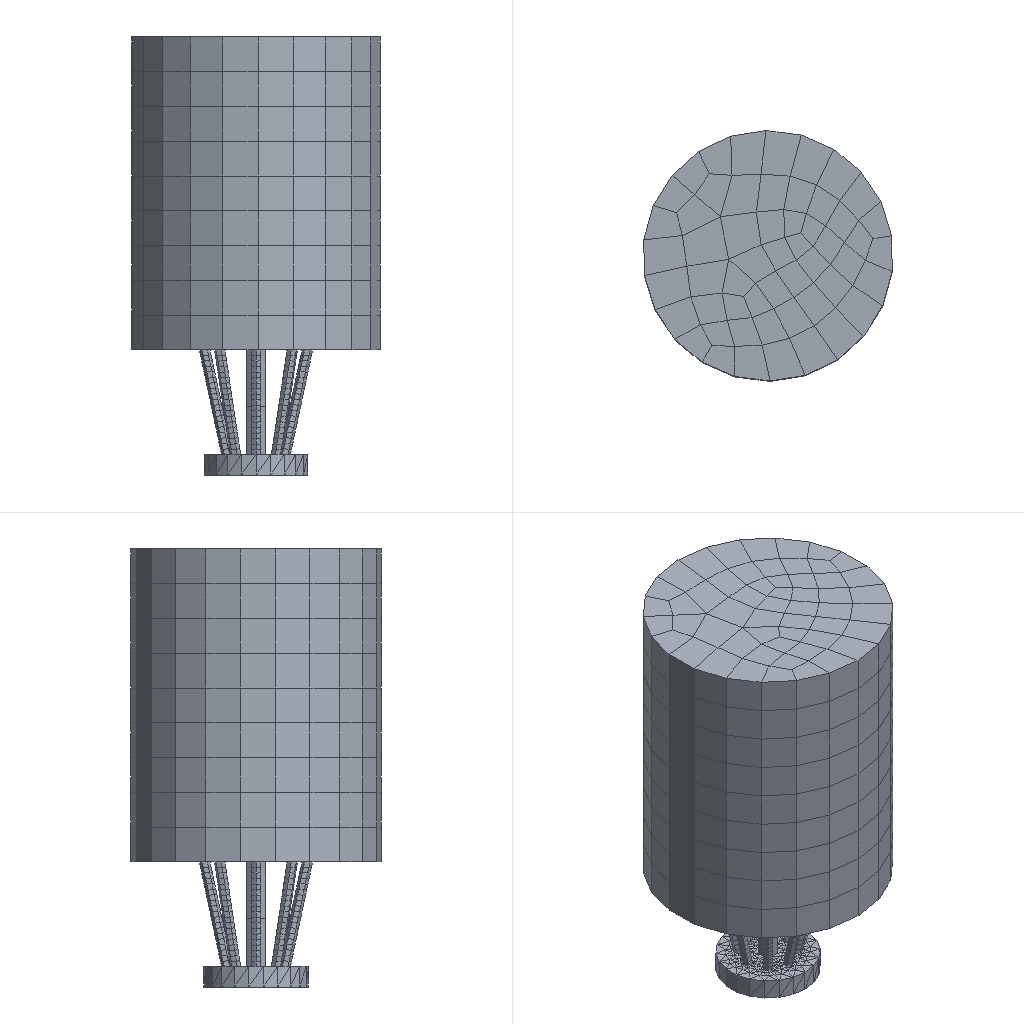Simulation study | abaqus
Set-up summary:
category,name,step,type,value,unit,region
solver,abaqus
solver,version,,,Abaqus/Standard 2020
units,not stated in the deck,,not stated
analysis,deck,,static,static
load_step,Step-1,Step-1,static
load_step,requested,,,1
mesh,nodes,,,8569
mesh,elements,,,4242
element_type,C3D8,,solid,1718
element_type,C3D10,,solid,2524
load,load commands in deck,,count,2
bc,support commands in deck,,count,3
material,CON,,in results
material,SOIL,,in results
check,setup vs results,,match,"per instance, exact: element labels, types and connectivity; labels of the nodes the elements use; coordinates of those nodes at SINGLE_PRECISION in 2 of 3 instance(s)"
Abaqus input file, long lists of numbers shortened:
*Heading
** Job name: Job-2 Model name: Model-2
** Generated by: Abaqus/CAE 2020
*Preprint, echo=NO, model=NO, history=NO, contact=NO
**
** PARTS
**
*Part, name=Part-3
*Node
      1,   3.383,  -3.971,          12.
      2,   1.788,  -2.376,   1.388
** (3727 more lines like these left out)
*Element, type=C3D8
 1, 174, 173, 172, 169,   1,  36,  35,  32
 2, 172, 171, 170, 169,  35,  34,  33,  32
** (1230 more lines like these left out)
*Nset, nset=Set-2, generate
    1,  3729,     1
*Elset, elset=Set-2, generate
    1,  1232,     1
** Section: con
*Solid Section, elset=Set-2, material=con
,
*End Part
**
*Part, name=cut-chengtai
*Node
      1,   1.788,  -2.376,   1.388
      2,  -2.376,  -1.788,   1.388
** (4178 more lines like these left out)
*Element, type=C3D10
   1,  398,  158,  399,  400,  634,  633,  632,  636,  635,  637
   2,  401,  402,  302,  403,  640,  639,  638,  642,  641,  643
** (2522 more lines like these left out)
*Nset, nset=Set-4, generate
    1,  4180,     1
*Elset, elset=Set-4, generate
    1,  2524,     1
** Section: con
*Solid Section, elset=Set-4, material=con
,
*End Part
**
*Part, name=soil
*Node
      1,   9.2,   -7.705,           0.
      2,   10.998,   -4.801,           0.
** (658 more lines like these left out)
*Element, type=C3D8
  1,  89,  86,  85,  90,  23,  20,  19,  24
  2,  90,  85,  84,  91,  24,  19,  18,  25
** (484 more lines like these left out)
*Nset, nset=Set-2, generate
   1,  660,    1
*Elset, elset=Set-2, generate
   1,  486,    1
** Section: soil
*Solid Section, elset=Set-2, material=soil
,
*End Part
**
**
** ASSEMBLY
**
*Assembly, name=Assembly
**
*Instance, name=soil-1, part=soil
          0.,           0.,          12.
*End Instance
**
*Instance, name=cut-chengtai-1, part=cut-chengtai
*End Instance
**
*Instance, name=Part-3-1, part=Part-3
*End Instance
**
*Nset, nset=Set-3, instance=soil-1, generate
 595,  660,    1
*Elset, elset=Set-3, instance=soil-1, generate
 433,  486,    1
*Nset, nset=Set-4, instance=soil-1
   1,   2,   3,   4,   5,   6,   7,   8,   9,  10,  11,  12,  13,  14,  15,  16
  17,  18,  19,  20,  21,  22,  67,  68,  69,  70,  71,  72,  73,  74,  75,  76
** (12 more lines like these left out)
*Elset, elset=Set-4, instance=soil-1
   1,   2,   3,   4,  13,  14,  15,  16,  17,  18,  19,  20,  22,  23,  24,  25
  26,  27,  28,  29,  48,  49,  55,  56,  57,  58,  67,  68,  69,  70,  71,  72
** (11 more lines like these left out)
*Nset, nset=Set-5, instance=soil-1, generate
 595,  660,    1
*Elset, elset=Set-5, instance=soil-1, generate
 433,  486,    1
*Nset, nset=m_Set-1, instance=Part-3-1
    1,    3,    4,    6,    7,   10,   11,   13,   14,   17,   18,   20,   21,   24,   25,   27
   28,   31,   32,   33,   34,   35,   36,   42,   43,   44,   45,   46,   47,   48,   49,   50
** (170 more lines like these left out)
*Elset, elset=m_Set-1, instance=Part-3-1
   41,   42,   43,   44,   45,   46,   47,   48,   49,   50,   51,   52,   53,   54,   55,   56
   57,   58,   59,   60,   61,   62,   63,   64,   65,   66,   67,   68,   69,   70,   71,   72
** (55 more lines like these left out)
*Nset, nset=s_Set-1, instance=soil-1, generate
   1,  660,    1
*Elset, elset=s_Set-1, instance=soil-1, generate
   1,  486,    1
*Elset, elset=_Surf-3_S1, internal, instance=cut-chengtai-1
  121, 1557, 1809
*Elset, elset=_Surf-3_S3, internal, instance=cut-chengtai-1
  487,  520,  610,  668,  694,  706,  761,  783,  858,  877,  881,  905,  949, 1073, 1092, 1116
 1209, 1248, 1259, 1293, 1321, 1361, 1389, 1441, 1450, 1472, 1490, 1537, 1539, 1556, 1562, 1566
** (3 more lines like these left out)
*Elset, elset=_Surf-3_S4, internal, instance=cut-chengtai-1
  587,  760, 1074, 1144, 1316, 1449, 1597, 1672, 2343
*Elset, elset=_Surf-3_S2, internal, instance=cut-chengtai-1
  673,  988, 1451, 1619, 1629, 1923, 2221, 2301
*Surface, type=ELEMENT, name=Surf-3
_Surf-3_S1, S1
_Surf-3_S3, S3
_Surf-3_S4, S4
_Surf-3_S2, S2
*Elset, elset=_Surf-4_S3, internal, instance=Part-3-1
    1,    2,    3,    4,    5,    6,    7,    8,    9,   10,   11,   12,   13,   14,   15,   16
   17,   18,   19,   20,   21,   22,   23,   24,   25,   26,   27,   28,   29,   30,   31,   32
** (19 more lines like these left out)
*Elset, elset=_Surf-4_S4, internal, instance=Part-3-1
    1,    2,    3,    4,    5,    6,    7,    8,    9,   10,   11,   12,   13,   14,   15,   16
   17,   18,   19,   20,   21,   22,   23,   24,   25,   26,   27,   28,   29,   30,   31,   32
** (14 more lines like these left out)
*Elset, elset=_Surf-4_S6, internal, instance=Part-3-1
    1,    3,    5,    7,    9,   11,   13,   15,   17,   19,   21,   23,   25,   27,   29,   31
   33,   35,   37,   39,  151,  153,  155,  157,  183,  184,  185,  186,  187,  188,  189,  190
** (14 more lines like these left out)
*Elset, elset=_Surf-4_S5, internal, instance=Part-3-1
    2,    4,    6,    8,   10,   12,   14,   16,   18,   20,   22,   24,   26,   28,   30,   32
   34,   36,   38,   40,  152,  154,  156,  158,  183,  185,  187,  189,  191,  193,  195,  197
** (9 more lines like these left out)
*Surface, type=ELEMENT, name=Surf-4
_Surf-4_S3, S3
_Surf-4_S4, S4
_Surf-4_S6, S6
_Surf-4_S5, S5
*Elset, elset=_m_Surf-1_S3, internal, instance=Part-3-1
    1,    2,    3,    4,    5,    6,    7,    8,    9,   10,   11,   12,   13,   14,   15,   16
   17,   18,   19,   20,   21,   22,   23,   24,   25,   26,   27,   28,   29,   30,   31,   32
** (19 more lines like these left out)
*Elset, elset=_m_Surf-1_S4, internal, instance=Part-3-1
    1,    2,    3,    4,    5,    6,    7,    8,    9,   10,   11,   12,   13,   14,   15,   16
   17,   18,   19,   20,   21,   22,   23,   24,   25,   26,   27,   28,   29,   30,   31,   32
** (14 more lines like these left out)
*Elset, elset=_m_Surf-1_S6, internal, instance=Part-3-1
    1,    3,    5,    7,    9,   11,   13,   15,   17,   19,   21,   23,   25,   27,   29,   31
   33,   35,   37,   39,  151,  153,  155,  157,  183,  184,  185,  186,  187,  188,  189,  190
** (14 more lines like these left out)
*Elset, elset=_m_Surf-1_S5, internal, instance=Part-3-1
    2,    4,    6,    8,   10,   12,   14,   16,   18,   20,   22,   24,   26,   28,   30,   32
   34,   36,   38,   40,  152,  154,  156,  158,  183,  185,  187,  189,  191,  193,  195,  197
** (9 more lines like these left out)
*Elset, elset=_m_Surf-1_S1, internal, instance=Part-3-1
   39,   40,  155,  156,  157,  158,  221,  222,  371,  372,  521,  522,  671,  672,  821,  822
  971,  972, 1121, 1122
*Surface, type=ELEMENT, name=m_Surf-1
_m_Surf-1_S3, S3
_m_Surf-1_S4, S4
_m_Surf-1_S6, S6
_m_Surf-1_S5, S5
_m_Surf-1_S1, S1
*Elset, elset=_s_Surf-1_S3, internal, instance=cut-chengtai-1
  128,  163,  233,  237,  241,  248,  251,  261,  271,  281,  288,  313,  343,  377,  389,  427
  490,  532,  544,  569,  604,  617,  851,  853,  985, 1075, 1179, 1253, 1306, 1386, 1518, 1538
** (12 more lines like these left out)
*Elset, elset=_s_Surf-1_S2, internal, instance=cut-chengtai-1
  229,  744,  778, 1056, 1759, 1942, 2086, 2088, 2103, 2184, 2234, 2262, 2288, 2326
*Elset, elset=_s_Surf-1_S4, internal, instance=cut-chengtai-1
  162,  280,  398, 1719, 1825, 1865, 1873, 2032, 2194
*Elset, elset=_s_Surf-1_S1, internal, instance=cut-chengtai-1
  884, 1120, 1401, 1981, 2136
*Surface, type=ELEMENT, name=s_Surf-1
_s_Surf-1_S3, S3
_s_Surf-1_S2, S2
_s_Surf-1_S4, S4
_s_Surf-1_S1, S1
** Constraint: Constraint-1
*Embedded Element, host elset=s_Set-1
m_Set-1
** Constraint: Constraint-2
*Tie, name=Constraint-2, adjust=yes
s_Surf-1, m_Surf-1
*End Assembly
*Amplitude, name=Amp-1
             0.,              0.,              1.,              1.
**
** MATERIALS
**
*Material, name=con
*Density
2770.,
*Elastic
 2.745e+10, 0.2
*Material, name=soil
*Density
2500.,
*Elastic
 1.3e+10, 0.35
**
** BOUNDARY CONDITIONS
**
** Name: BC-2 Type: 位移/转角
*Boundary
Set-4, 1, 1
Set-4, 2, 2
** Name: BC-3 Type: 位移/转角
*Boundary
Set-5, 3, 3
** ----------------------------------------------------------------
**
** STEP: Step-1
**
*Step, name=Step-1, nlgeom=YES, inc=1000
*Static, stabilize=0.0002, allsdtol=0.05, continue=NO
0.001, 1., 1e-05, 1.
**
** LOADS
**
** Name: Load-1   Type: Pressure
*Dsload, amplitude=Amp-1
Surf-3, P, 10.
** Name: Load-2   Type: Surface traction
*Dsload, amplitude=Amp-1
Surf-4, TRVEC, 10., 0., 1., 0.
**
** OUTPUT REQUESTS
**
*Restart, write, frequency=0
**
** FIELD OUTPUT: F-Output-1
**
*Output, field
*Node Output
CF, RF, U
*Element Output, directions=YES
E, LE, MISES, PE, PEEQ, PEMAG, S
*Contact Output
CDISP, CSTRESS
**
** HISTORY OUTPUT: H-Output-1
**
*Output, history, variable=PRESELECT
*End Step
Results summary:
result,step,,completed,increments=17 time=1.0/1.0
result,analysis,,,static
result,last_loadstep,,,1
result,primary field,,,U
result,reaction total,,FX,-0.000335,model units
result,reaction total,,FY,-3250.713,model units
result,reaction total,,FZ,-785.385,model units